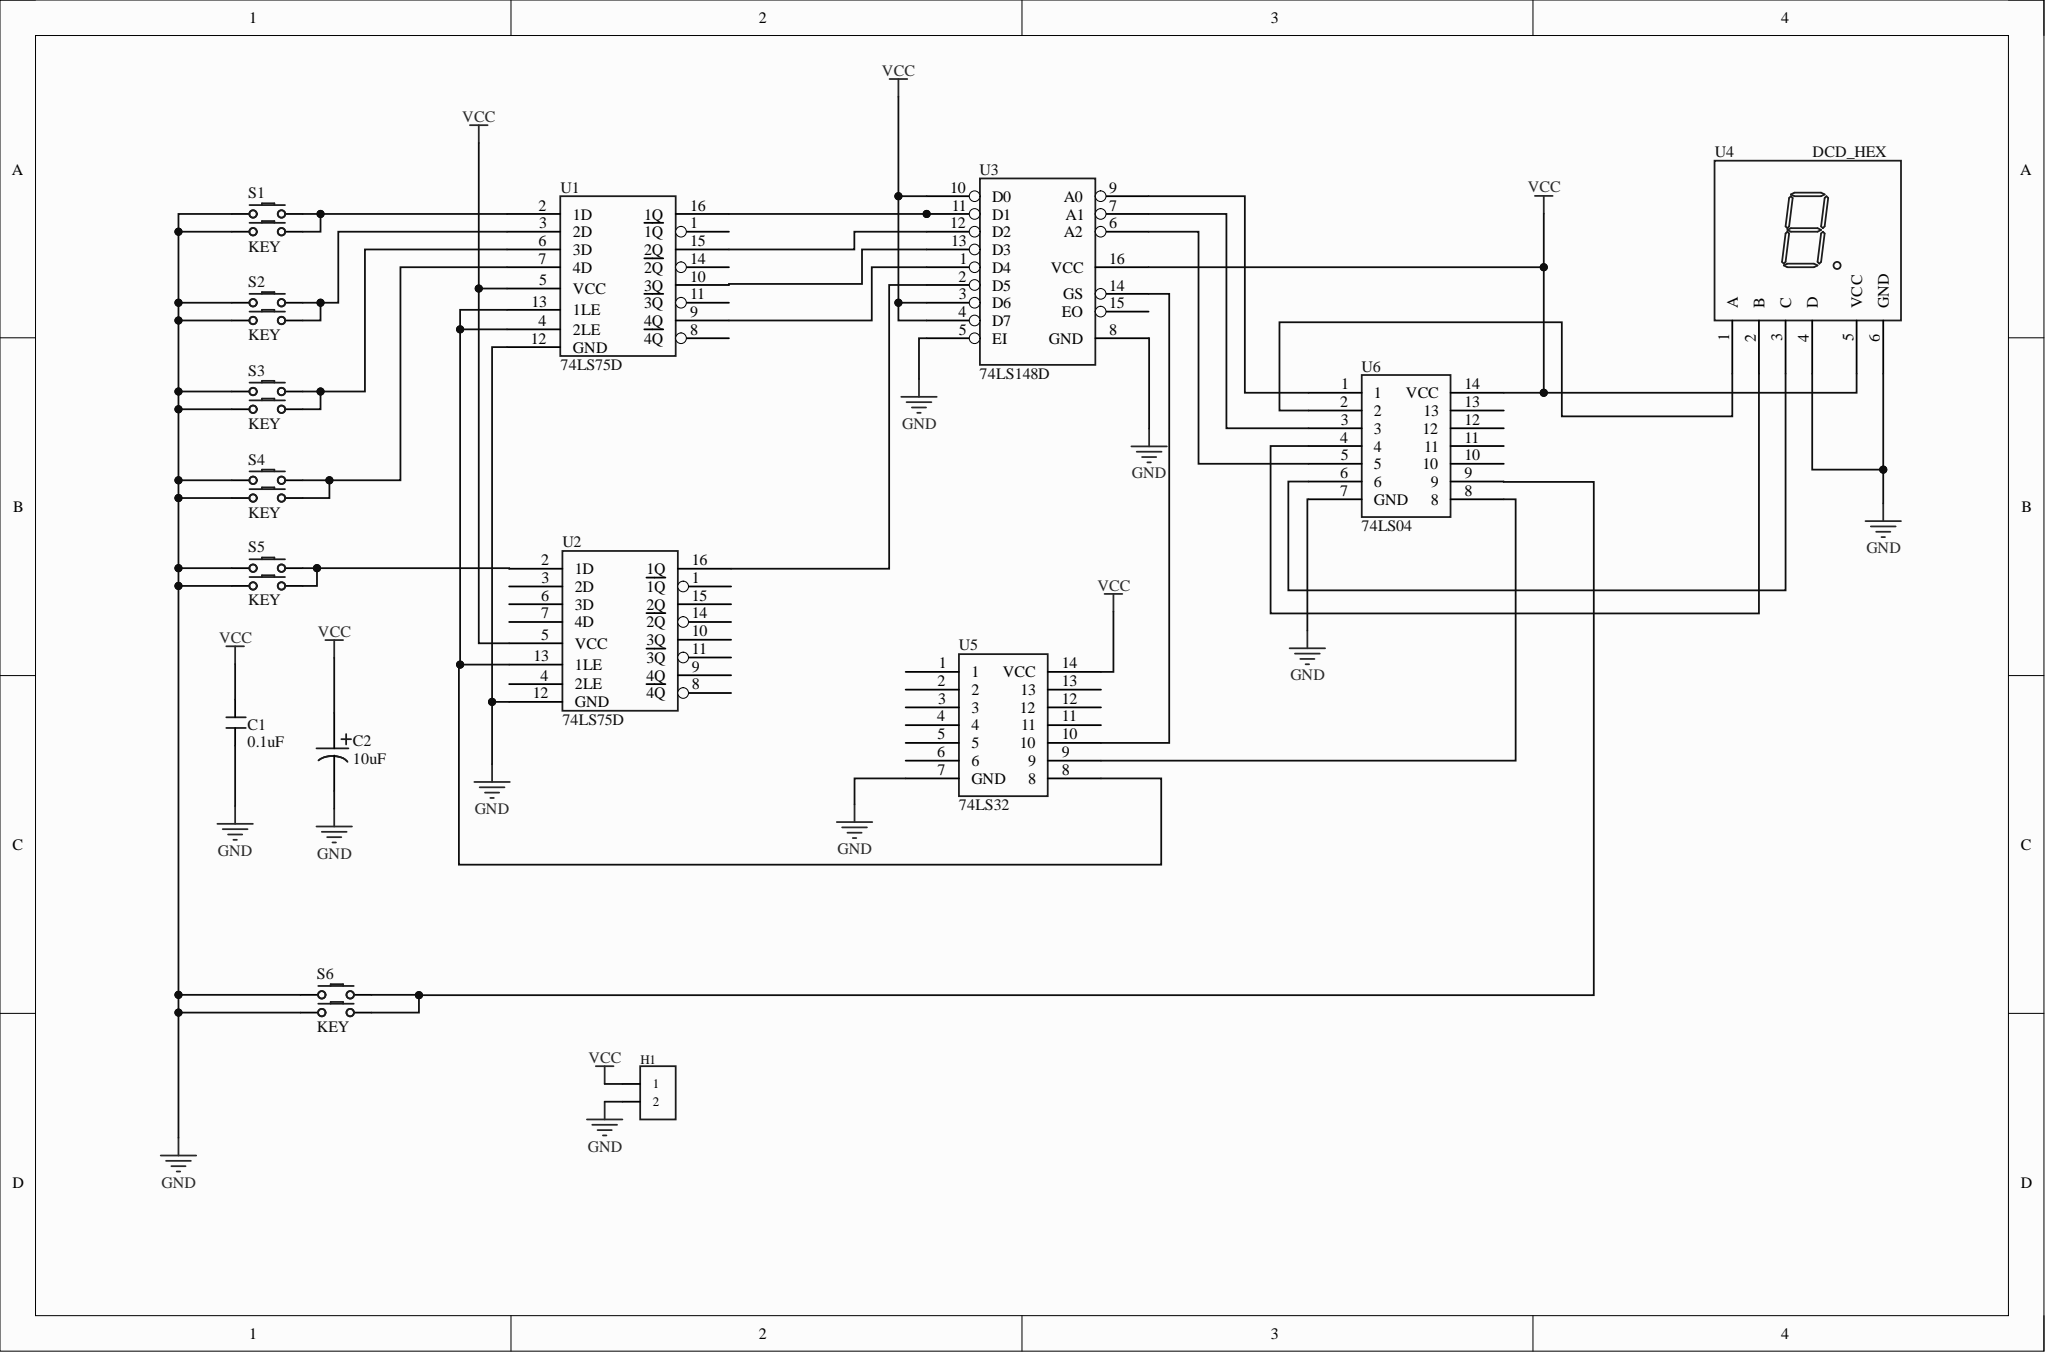Circuit board | Altium Designer | 15 parts | 22 nets
Bill of materials:
Comment,Description,Designator,Footprint,LibRef,Quantity
"0.1uF","","C1","CAP","Cap","1"
"10uF","","C2","CAP POL","Cap Pol","1"
"","","H1","HDR-TH_2P-P2.54-V-F","HDR-F_2.54_1x2P","1"
"KEY","","S1, S2, S3, S4, S5, S6","KEY-4","KEY-4","6"
"74LS75D","","U1, U2","74LS75D","74LS75D","2"
"74LS148D","","U3","74LS148D","74LS148D","1"
"DCD_HEX","","U4","SMG","SMG","1"
"74LS32","","U5","74LS32","74LS32","1"
"74LS04","","U6","74LS04","74LS04","1"
Netlist (Protel format):
[
C1
CAP
0.1uF



]
[
C2
CAP POL
10uF



]
[
H1
HDR-TH_2P-P2.54-V-F




]
[
S1
KEY-4
KEY



]
[
S2
KEY-4
KEY



]
[
S3
KEY-4
KEY



]
[
S4
KEY-4
KEY



]
[
S5
KEY-4
KEY



]
[
S6
KEY-4
KEY



]
[
U1
74LS75D
74LS75D



]
[
U2
74LS75D
74LS75D



]
[
U3
74LS148D
74LS148D



]
[
U4
SMG
DCD_HEX



]
[
U5
74LS32
74LS32



]
[
U6
74LS04
74LS04



]
(
VCC
C1-2
C2-1
H1-1
U1-5
U2-5
U3-3
U3-4
U3-10
U3-16
U4-5
U5-14
U6-14
)
(
NetU5_9
U5-9
U6-8
)
(
NetU4_3
U4-3
U6-6
)
(
NetU4_2
U4-2
U6-4
)
(
NetU4_1
U4-1
U6-2
)
(
NetU3_14
U3-14
U5-10
)
(
NetU3_9
U3-9
U6-1
)
(
NetU3_7
U3-7
U6-3
)
(
NetU3_6
U3-6
U6-5
)
(
NetU2_16
U2-16
U3-2
)
(
NetU1_16
U1-16
U3-11
)
(
NetU1_15
U1-15
U3-12
)
(
NetU1_10
U1-10
U3-13
)
(
NetU1_9
U1-9
U3-1
)
(
NetU1_4
U1-4
U1-13
U2-13
U5-8
)
(
NetS6_2
S6-2
S6-4
U6-9
)
(
NetS5_2
S5-2
S5-4
U2-2
)
(
NetS4_2
S4-2
S4-4
U1-7
)
(
NetS3_2
S3-2
S3-4
U1-6
)
(
NetS2_2
S2-2
S2-4
U1-3
)
(
NetS1_2
S1-2
S1-4
U1-2
)
(
GND
C1-1
C2-2
H1-2
S1-1
S1-3
S2-1
S2-3
S3-1
S3-3
S4-1
S4-3
S5-1
S5-3
S6-1
S6-3
U1-12
U2-12
U3-5
U3-8
U4-4
U4-6
U5-7
U6-7
)